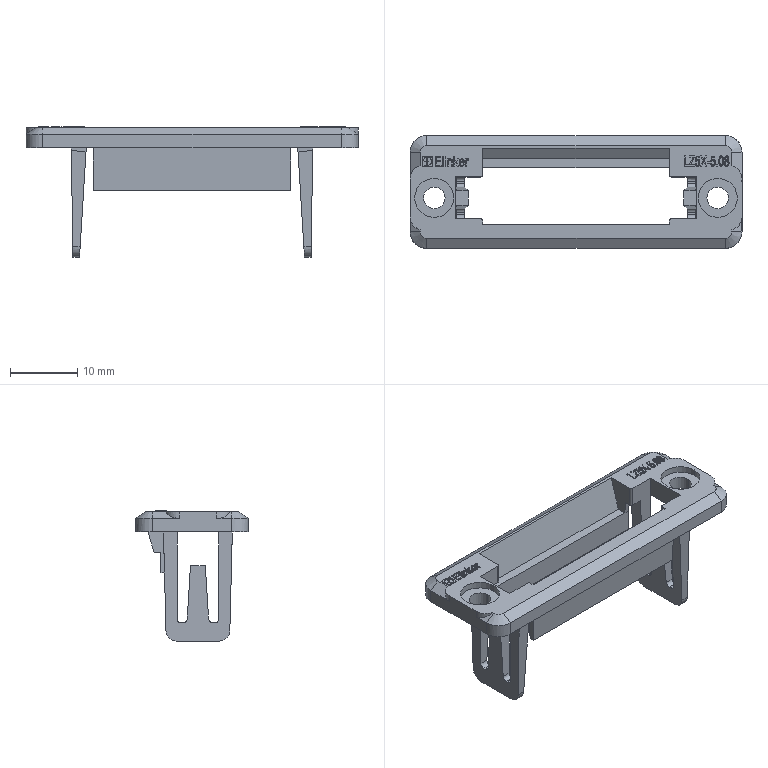Part | NX | features BREP 1 | 1 solid | 1088 faces | box 49.28 x 16.75 x 19.3 mm | volume 1912 mm3 | plane 990 | spline 52 | cylinder 42 | cone 4 | commonest cylinder face diameters 1.2 x8 3.2 x8 0.252 x4 0.6 x4 4.035 x4 5 x4